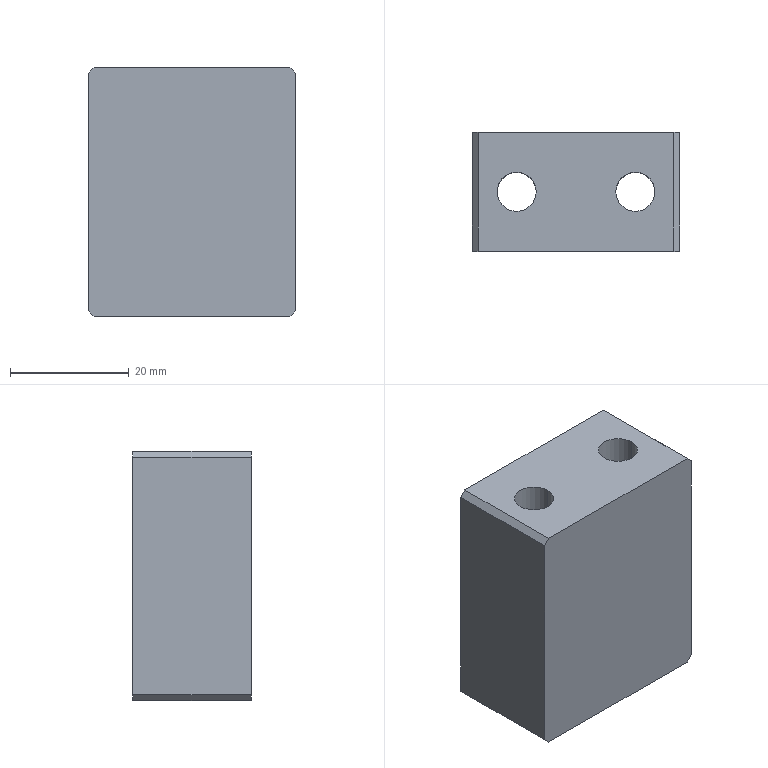Part | SolidWorks | features BaseBody 1 | 1 solid | 20 faces | box 35 x 20 x 42 mm | volume 25659 mm3 | plane 12 | cylinder 8 | commonest cylinder face diameters 6.6 x4 11 x4
STEP:
#1=CARTESIAN_POINT('',(-16.5,10.,-21.));
#2=VERTEX_POINT('',#1);
#3=CARTESIAN_POINT('',(-17.5,10.,-20.));
#4=VERTEX_POINT('',#3);
#5=CARTESIAN_POINT('',(-17.5,10.,-20.));
#6=DIRECTION('',(-0.7071,0.,0.7071));
#7=VECTOR('',#6,1000.);
#8=LINE('',#5,#7);
#9=EDGE_CURVE('',#2,#4,#8,.T.);
#10=ORIENTED_EDGE('',*,*,#9,.F.);
#11=CARTESIAN_POINT('',(-16.5,-10.,-21.));
#12=VERTEX_POINT('',#11);
#13=CARTESIAN_POINT('',(-16.5,10.,-21.));
#14=DIRECTION('',(0.,1.,0.));
#15=VECTOR('',#14,1000.);
#16=LINE('',#13,#15);
#17=EDGE_CURVE('',#12,#2,#16,.T.);
#18=ORIENTED_EDGE('',*,*,#17,.F.);
#19=CARTESIAN_POINT('',(-17.5,-10.,-20.));
#20=VERTEX_POINT('',#19);
#21=CARTESIAN_POINT('',(-18.75,-10.,-18.75));
#22=DIRECTION('',(0.7071,0.,-0.7071));
#23=VECTOR('',#22,1000.);
#24=LINE('',#21,#23);
#25=EDGE_CURVE('',#20,#12,#24,.T.);
#26=ORIENTED_EDGE('',*,*,#25,.F.);
#27=CARTESIAN_POINT('',(-17.5,10.,-20.));
#28=DIRECTION('',(0.,-1.,0.));
#29=VECTOR('',#28,1000.);
#30=LINE('',#27,#29);
#31=EDGE_CURVE('',#4,#20,#30,.T.);
#32=ORIENTED_EDGE('',*,*,#31,.F.);
#33=EDGE_LOOP('',(#10,#18,#26,#32));
#34=FACE_OUTER_BOUND('',#33,.T.);
#35=CARTESIAN_POINT('',(-17.5,10.,-20.));
#36=DIRECTION('',(0.7071,0.,0.7071));
#37=DIRECTION('',(0.,-1.,0.));
#38=AXIS2_PLACEMENT_3D('',#35,#36,#37);
#39=PLANE('',#38);
#40=ADVANCED_FACE('',(#34),#39,.F.);
#41=CARTESIAN_POINT('',(17.5,10.,-20.));
#42=VERTEX_POINT('',#41);
#43=CARTESIAN_POINT('',(16.5,10.,-21.));
#44=VERTEX_POINT('',#43);
#45=CARTESIAN_POINT('',(16.5,10.,-21.));
#46=DIRECTION('',(-0.7071,0.,-0.7071));
#47=VECTOR('',#46,1000.);
#48=LINE('',#45,#47);
#49=EDGE_CURVE('',#42,#44,#48,.T.);
#50=ORIENTED_EDGE('',*,*,#49,.F.);
#51=CARTESIAN_POINT('',(17.5,-10.,-20.));
#52=VERTEX_POINT('',#51);
#53=CARTESIAN_POINT('',(17.5,10.,-20.));
#54=DIRECTION('',(0.,1.,0.));
#55=VECTOR('',#54,1000.);
#56=LINE('',#53,#55);
#57=EDGE_CURVE('',#52,#42,#56,.T.);
#58=ORIENTED_EDGE('',*,*,#57,.F.);
#59=CARTESIAN_POINT('',(16.5,-10.,-21.));
#60=VERTEX_POINT('',#59);
#61=CARTESIAN_POINT('',(18.75,-10.,-18.75));
#62=DIRECTION('',(0.7071,0.,0.7071));
#63=VECTOR('',#62,1000.);
#64=LINE('',#61,#63);
#65=EDGE_CURVE('',#60,#52,#64,.T.);
#66=ORIENTED_EDGE('',*,*,#65,.F.);
#67=CARTESIAN_POINT('',(16.5,10.,-21.));
#68=DIRECTION('',(0.,-1.,0.));
#69=VECTOR('',#68,1000.);
#70=LINE('',#67,#69);
#71=EDGE_CURVE('',#44,#60,#70,.T.);
#72=ORIENTED_EDGE('',*,*,#71,.F.);
#73=EDGE_LOOP('',(#50,#58,#66,#72));
#74=FACE_OUTER_BOUND('',#73,.T.);
#75=CARTESIAN_POINT('',(16.5,10.,-21.));
#76=DIRECTION('',(-0.7071,0.,0.7071));
#77=DIRECTION('',(0.,1.,0.));
#78=AXIS2_PLACEMENT_3D('',#75,#76,#77);
#79=PLANE('',#78);
#80=ADVANCED_FACE('',(#74),#79,.F.);
#81=CARTESIAN_POINT('',(-17.5,10.,20.));
#82=VERTEX_POINT('',#81);
#83=CARTESIAN_POINT('',(-16.5,10.,21.));
#84=VERTEX_POINT('',#83);
#85=CARTESIAN_POINT('',(-16.5,10.,21.));
#86=DIRECTION('',(0.7071,0.,0.7071));
#87=VECTOR('',#86,1000.);
#88=LINE('',#85,#87);
#89=EDGE_CURVE('',#82,#84,#88,.T.);
#90=ORIENTED_EDGE('',*,*,#89,.F.);
#91=CARTESIAN_POINT('',(-17.5,-10.,20.));
#92=VERTEX_POINT('',#91);
#93=CARTESIAN_POINT('',(-17.5,10.,20.));
#94=DIRECTION('',(0.,1.,0.));
#95=VECTOR('',#94,1000.);
#96=LINE('',#93,#95);
#97=EDGE_CURVE('',#92,#82,#96,.T.);
#98=ORIENTED_EDGE('',*,*,#97,.F.);
#99=CARTESIAN_POINT('',(-16.5,-10.,21.));
#100=VERTEX_POINT('',#99);
#101=CARTESIAN_POINT('',(-18.75,-10.,18.75));
#102=DIRECTION('',(-0.7071,0.,-0.7071));
#103=VECTOR('',#102,1000.);
#104=LINE('',#101,#103);
#105=EDGE_CURVE('',#100,#92,#104,.T.);
#106=ORIENTED_EDGE('',*,*,#105,.F.);
#107=CARTESIAN_POINT('',(-16.5,10.,21.));
#108=DIRECTION('',(0.,-1.,0.));
#109=VECTOR('',#108,1000.);
#110=LINE('',#107,#109);
#111=EDGE_CURVE('',#84,#100,#110,.T.);
#112=ORIENTED_EDGE('',*,*,#111,.F.);
#113=EDGE_LOOP('',(#90,#98,#106,#112));
#114=FACE_OUTER_BOUND('',#113,.T.);
#115=CARTESIAN_POINT('',(-16.5,10.,21.));
#116=DIRECTION('',(0.7071,0.,-0.7071));
#117=DIRECTION('',(0.,-1.,0.));
#118=AXIS2_PLACEMENT_3D('',#115,#116,#117);
#119=PLANE('',#118);
#120=ADVANCED_FACE('',(#114),#119,.F.);
#121=CARTESIAN_POINT('',(16.5,10.,21.));
#122=VERTEX_POINT('',#121);
#123=CARTESIAN_POINT('',(17.5,10.,20.));
#124=VERTEX_POINT('',#123);
#125=CARTESIAN_POINT('',(17.5,10.,20.));
#126=DIRECTION('',(0.7071,0.,-0.7071));
#127=VECTOR('',#126,1000.);
#128=LINE('',#125,#127);
#129=EDGE_CURVE('',#122,#124,#128,.T.);
#130=ORIENTED_EDGE('',*,*,#129,.F.);
#131=CARTESIAN_POINT('',(16.5,-10.,21.));
#132=VERTEX_POINT('',#131);
#133=CARTESIAN_POINT('',(16.5,10.,21.));
#134=DIRECTION('',(0.,1.,0.));
#135=VECTOR('',#134,1000.);
#136=LINE('',#133,#135);
#137=EDGE_CURVE('',#132,#122,#136,.T.);
#138=ORIENTED_EDGE('',*,*,#137,.F.);
#139=CARTESIAN_POINT('',(17.5,-10.,20.));
#140=VERTEX_POINT('',#139);
#141=CARTESIAN_POINT('',(18.75,-10.,18.75));
#142=DIRECTION('',(-0.7071,0.,0.7071));
#143=VECTOR('',#142,1000.);
#144=LINE('',#141,#143);
#145=EDGE_CURVE('',#140,#132,#144,.T.);
#146=ORIENTED_EDGE('',*,*,#145,.F.);
#147=CARTESIAN_POINT('',(17.5,10.,20.));
#148=DIRECTION('',(0.,-1.,0.));
#149=VECTOR('',#148,1000.);
#150=LINE('',#147,#149);
#151=EDGE_CURVE('',#124,#140,#150,.T.);
#152=ORIENTED_EDGE('',*,*,#151,.F.);
#153=EDGE_LOOP('',(#130,#138,#146,#152));
#154=FACE_OUTER_BOUND('',#153,.T.);
#155=CARTESIAN_POINT('',(17.5,10.,20.));
#156=DIRECTION('',(-0.7071,0.,-0.7071));
#157=DIRECTION('',(-0.7071,0.,0.7071));
#158=AXIS2_PLACEMENT_3D('',#155,#156,#157);
#159=PLANE('',#158);
#160=ADVANCED_FACE('',(#154),#159,.F.);
#161=CARTESIAN_POINT('',(-4.5,0.,-14.2));
#162=VERTEX_POINT('',#161);
#163=CARTESIAN_POINT('',(-4.5,0.,-21.));
#164=VERTEX_POINT('',#163);
#165=CARTESIAN_POINT('',(-4.5,0.,-21.));
#166=DIRECTION('',(0.,0.,-1.));
#167=VECTOR('',#166,1000.);
#168=LINE('',#165,#167);
#169=EDGE_CURVE('',#162,#164,#168,.T.);
#170=ORIENTED_EDGE('',*,*,#169,.F.);
#171=CARTESIAN_POINT('',(-15.5,0.,-14.2));
#172=VERTEX_POINT('',#171);
#173=CARTESIAN_POINT('',(-10.,0.,-14.2));
#174=DIRECTION('',(0.,0.,-1.));
#175=DIRECTION('',(-1.,0.,0.));
#176=AXIS2_PLACEMENT_3D('',#173,#174,#175);
#177=CIRCLE('',#176,5.5);
#178=EDGE_CURVE('',#172,#162,#177,.T.);
#179=ORIENTED_EDGE('',*,*,#178,.F.);
#180=CARTESIAN_POINT('',(-15.5,0.,-21.));
#181=VERTEX_POINT('',#180);
#182=CARTESIAN_POINT('',(-15.5,0.,-21.));
#183=DIRECTION('',(0.,0.,-1.));
#184=VECTOR('',#183,1000.);
#185=LINE('',#182,#184);
#186=EDGE_CURVE('',#172,#181,#185,.T.);
#187=ORIENTED_EDGE('',*,*,#186,.T.);
#188=CARTESIAN_POINT('',(-10.,0.,-21.));
#189=DIRECTION('',(0.,0.,-1.));
#190=DIRECTION('',(-1.,0.,0.));
#191=AXIS2_PLACEMENT_3D('',#188,#189,#190);
#192=CIRCLE('',#191,5.5);
#193=EDGE_CURVE('',#181,#164,#192,.T.);
#194=ORIENTED_EDGE('',*,*,#193,.T.);
#195=EDGE_LOOP('',(#170,#179,#187,#194));
#196=FACE_OUTER_BOUND('',#195,.T.);
#197=CARTESIAN_POINT('',(-10.,0.,-21.));
#198=DIRECTION('',(0.,0.,-1.));
#199=DIRECTION('',(-1.,0.,0.));
#200=AXIS2_PLACEMENT_3D('',#197,#198,#199);
#201=CYLINDRICAL_SURFACE('',#200,5.5);
#202=ADVANCED_FACE('',(#196),#201,.F.);
#203=CARTESIAN_POINT('',(-13.3,0.,-14.2));
#204=VERTEX_POINT('',#203);
#205=CARTESIAN_POINT('',(-6.7,0.,-14.2));
#206=VERTEX_POINT('',#205);
#207=CARTESIAN_POINT('',(-10.,0.,-14.2));
#208=DIRECTION('',(0.,0.,-1.));
#209=DIRECTION('',(-1.,0.,0.));
#210=AXIS2_PLACEMENT_3D('',#207,#208,#209);
#211=CIRCLE('',#210,3.3);
#212=EDGE_CURVE('',#204,#206,#211,.T.);
#213=ORIENTED_EDGE('',*,*,#212,.F.);
#214=CARTESIAN_POINT('',(-10.,0.,-14.2));
#215=DIRECTION('',(0.,0.,-1.));
#216=DIRECTION('',(-1.,0.,0.));
#217=AXIS2_PLACEMENT_3D('',#214,#215,#216);
#218=CIRCLE('',#217,3.3);
#219=EDGE_CURVE('',#206,#204,#218,.T.);
#220=ORIENTED_EDGE('',*,*,#219,.F.);
#221=EDGE_LOOP('',(#213,#220));
#222=FACE_BOUND('',#221,.T.);
#223=ORIENTED_EDGE('',*,*,#178,.T.);
#224=CARTESIAN_POINT('',(-10.,0.,-14.2));
#225=DIRECTION('',(0.,0.,-1.));
#226=DIRECTION('',(-1.,0.,0.));
#227=AXIS2_PLACEMENT_3D('',#224,#225,#226);
#228=CIRCLE('',#227,5.5);
#229=EDGE_CURVE('',#162,#172,#228,.T.);
#230=ORIENTED_EDGE('',*,*,#229,.T.);
#231=EDGE_LOOP('',(#223,#230));
#232=FACE_OUTER_BOUND('',#231,.T.);
#233=CARTESIAN_POINT('',(-6.7,0.,-14.2));
#234=DIRECTION('',(0.,0.,1.));
#235=DIRECTION('',(1.,0.,0.));
#236=AXIS2_PLACEMENT_3D('',#233,#234,#235);
#237=PLANE('',#236);
#238=ADVANCED_FACE('',(#222,#232),#237,.F.);
#239=CARTESIAN_POINT('',(-6.7,0.,21.));
#240=VERTEX_POINT('',#239);
#241=CARTESIAN_POINT('',(-6.7,0.,-21.));
#242=DIRECTION('',(0.,0.,-1.));
#243=VECTOR('',#242,1000.);
#244=LINE('',#241,#243);
#245=EDGE_CURVE('',#240,#206,#244,.T.);
#246=ORIENTED_EDGE('',*,*,#245,.F.);
#247=CARTESIAN_POINT('',(-13.3,0.,21.));
#248=VERTEX_POINT('',#247);
#249=CARTESIAN_POINT('',(-10.,0.,21.));
#250=DIRECTION('',(0.,0.,-1.));
#251=DIRECTION('',(-1.,0.,0.));
#252=AXIS2_PLACEMENT_3D('',#249,#250,#251);
#253=CIRCLE('',#252,3.3);
#254=EDGE_CURVE('',#248,#240,#253,.T.);
#255=ORIENTED_EDGE('',*,*,#254,.F.);
#256=CARTESIAN_POINT('',(-13.3,0.,-21.));
#257=DIRECTION('',(0.,0.,-1.));
#258=VECTOR('',#257,1000.);
#259=LINE('',#256,#258);
#260=EDGE_CURVE('',#248,#204,#259,.T.);
#261=ORIENTED_EDGE('',*,*,#260,.T.);
#262=ORIENTED_EDGE('',*,*,#212,.T.);
#263=EDGE_LOOP('',(#246,#255,#261,#262));
#264=FACE_OUTER_BOUND('',#263,.T.);
#265=CARTESIAN_POINT('',(-10.,0.,-21.));
#266=DIRECTION('',(0.,0.,-1.));
#267=DIRECTION('',(-1.,0.,0.));
#268=AXIS2_PLACEMENT_3D('',#265,#266,#267);
#269=CYLINDRICAL_SURFACE('',#268,3.3);
#270=ADVANCED_FACE('',(#264),#269,.F.);
#271=CARTESIAN_POINT('',(15.5,0.,-14.2));
#272=VERTEX_POINT('',#271);
#273=CARTESIAN_POINT('',(15.5,0.,-21.));
#274=VERTEX_POINT('',#273);
#275=CARTESIAN_POINT('',(15.5,0.,-21.));
#276=DIRECTION('',(0.,0.,-1.));
#277=VECTOR('',#276,1000.);
#278=LINE('',#275,#277);
#279=EDGE_CURVE('',#272,#274,#278,.T.);
#280=ORIENTED_EDGE('',*,*,#279,.F.);
#281=CARTESIAN_POINT('',(4.5,0.,-14.2));
#282=VERTEX_POINT('',#281);
#283=CARTESIAN_POINT('',(10.,0.,-14.2));
#284=DIRECTION('',(0.,0.,-1.));
#285=DIRECTION('',(-1.,0.,0.));
#286=AXIS2_PLACEMENT_3D('',#283,#284,#285);
#287=CIRCLE('',#286,5.5);
#288=EDGE_CURVE('',#282,#272,#287,.T.);
#289=ORIENTED_EDGE('',*,*,#288,.F.);
#290=CARTESIAN_POINT('',(4.5,0.,-21.));
#291=VERTEX_POINT('',#290);
#292=CARTESIAN_POINT('',(4.5,0.,-21.));
#293=DIRECTION('',(0.,0.,-1.));
#294=VECTOR('',#293,1000.);
#295=LINE('',#292,#294);
#296=EDGE_CURVE('',#282,#291,#295,.T.);
#297=ORIENTED_EDGE('',*,*,#296,.T.);
#298=CARTESIAN_POINT('',(10.,0.,-21.));
#299=DIRECTION('',(0.,0.,-1.));
#300=DIRECTION('',(-1.,0.,0.));
#301=AXIS2_PLACEMENT_3D('',#298,#299,#300);
#302=CIRCLE('',#301,5.5);
#303=EDGE_CURVE('',#291,#274,#302,.T.);
#304=ORIENTED_EDGE('',*,*,#303,.T.);
#305=EDGE_LOOP('',(#280,#289,#297,#304));
#306=FACE_OUTER_BOUND('',#305,.T.);
#307=CARTESIAN_POINT('',(10.,0.,-21.));
#308=DIRECTION('',(0.,0.,-1.));
#309=DIRECTION('',(-1.,0.,0.));
#310=AXIS2_PLACEMENT_3D('',#307,#308,#309);
#311=CYLINDRICAL_SURFACE('',#310,5.5);
#312=ADVANCED_FACE('',(#306),#311,.F.);
#313=CARTESIAN_POINT('',(6.7,0.,-14.2));
#314=VERTEX_POINT('',#313);
#315=CARTESIAN_POINT('',(13.3,0.,-14.2));
#316=VERTEX_POINT('',#315);
#317=CARTESIAN_POINT('',(10.,0.,-14.2));
#318=DIRECTION('',(0.,0.,-1.));
#319=DIRECTION('',(-1.,0.,0.));
#320=AXIS2_PLACEMENT_3D('',#317,#318,#319);
#321=CIRCLE('',#320,3.3);
#322=EDGE_CURVE('',#314,#316,#321,.T.);
#323=ORIENTED_EDGE('',*,*,#322,.F.);
#324=CARTESIAN_POINT('',(10.,0.,-14.2));
#325=DIRECTION('',(0.,0.,-1.));
#326=DIRECTION('',(-1.,0.,0.));
#327=AXIS2_PLACEMENT_3D('',#324,#325,#326);
#328=CIRCLE('',#327,3.3);
#329=EDGE_CURVE('',#316,#314,#328,.T.);
#330=ORIENTED_EDGE('',*,*,#329,.F.);
#331=EDGE_LOOP('',(#323,#330));
#332=FACE_BOUND('',#331,.T.);
#333=ORIENTED_EDGE('',*,*,#288,.T.);
#334=CARTESIAN_POINT('',(10.,0.,-14.2));
#335=DIRECTION('',(0.,0.,-1.));
#336=DIRECTION('',(-1.,0.,0.));
#337=AXIS2_PLACEMENT_3D('',#334,#335,#336);
#338=CIRCLE('',#337,5.5);
#339=EDGE_CURVE('',#272,#282,#338,.T.);
#340=ORIENTED_EDGE('',*,*,#339,.T.);
#341=EDGE_LOOP('',(#333,#340));
#342=FACE_OUTER_BOUND('',#341,.T.);
#343=CARTESIAN_POINT('',(13.3,0.,-14.2));
#344=DIRECTION('',(0.,0.,1.));
#345=DIRECTION('',(1.,0.,0.));
#346=AXIS2_PLACEMENT_3D('',#343,#344,#345);
#347=PLANE('',#346);
#348=ADVANCED_FACE('',(#332,#342),#347,.F.);
#349=CARTESIAN_POINT('',(13.3,0.,21.));
#350=VERTEX_POINT('',#349);
#351=CARTESIAN_POINT('',(13.3,0.,-21.));
#352=DIRECTION('',(0.,0.,-1.));
#353=VECTOR('',#352,1000.);
#354=LINE('',#351,#353);
#355=EDGE_CURVE('',#350,#316,#354,.T.);
#356=ORIENTED_EDGE('',*,*,#355,.F.);
#357=CARTESIAN_POINT('',(6.7,0.,21.));
#358=VERTEX_POINT('',#357);
#359=CARTESIAN_POINT('',(10.,0.,21.));
#360=DIRECTION('',(0.,0.,-1.));
#361=DIRECTION('',(-1.,0.,0.));
#362=AXIS2_PLACEMENT_3D('',#359,#360,#361);
#363=CIRCLE('',#362,3.3);
#364=EDGE_CURVE('',#358,#350,#363,.T.);
#365=ORIENTED_EDGE('',*,*,#364,.F.);
#366=CARTESIAN_POINT('',(6.7,0.,-21.));
#367=DIRECTION('',(0.,0.,-1.));
#368=VECTOR('',#367,1000.);
#369=LINE('',#366,#368);
#370=EDGE_CURVE('',#358,#314,#369,.T.);
#371=ORIENTED_EDGE('',*,*,#370,.T.);
#372=ORIENTED_EDGE('',*,*,#322,.T.);
#373=EDGE_LOOP('',(#356,#365,#371,#372));
#374=FACE_OUTER_BOUND('',#373,.T.);
#375=CARTESIAN_POINT('',(10.,0.,-21.));
#376=DIRECTION('',(0.,0.,-1.));
#377=DIRECTION('',(-1.,0.,0.));
#378=AXIS2_PLACEMENT_3D('',#375,#376,#377);
#379=CYLINDRICAL_SURFACE('',#378,3.3);
#380=ADVANCED_FACE('',(#374),#379,.F.);
#381=CARTESIAN_POINT('',(17.5,-10.,21.));
#382=DIRECTION('',(0.,0.,-1.));
#383=VECTOR('',#382,1000.);
#384=LINE('',#381,#383);
#385=EDGE_CURVE('',#140,#52,#384,.T.);
#386=ORIENTED_EDGE('',*,*,#385,.F.);
#387=ORIENTED_EDGE('',*,*,#145,.T.);
#388=CARTESIAN_POINT('',(-17.5,-10.,21.));
#389=DIRECTION('',(1.,0.,0.));
#390=VECTOR('',#389,1000.);
#391=LINE('',#388,#390);
#392=EDGE_CURVE('',#100,#132,#391,.T.);
#393=ORIENTED_EDGE('',*,*,#392,.F.);
#394=ORIENTED_EDGE('',*,*,#105,.T.);
#395=CARTESIAN_POINT('',(-17.5,-10.,21.));
#396=DIRECTION('',(0.,0.,1.));
#397=VECTOR('',#396,1000.);
#398=LINE('',#395,#397);
#399=EDGE_CURVE('',#20,#92,#398,.T.);
#400=ORIENTED_EDGE('',*,*,#399,.F.);
#401=ORIENTED_EDGE('',*,*,#25,.T.);
#402=CARTESIAN_POINT('',(-17.5,-10.,-21.));
#403=DIRECTION('',(-1.,0.,0.));
#404=VECTOR('',#403,1000.);
#405=LINE('',#402,#404);
#406=EDGE_CURVE('',#60,#12,#405,.T.);
#407=ORIENTED_EDGE('',*,*,#406,.F.);
#408=ORIENTED_EDGE('',*,*,#65,.T.);
#409=EDGE_LOOP('',(#386,#387,#393,#394,#400,#401,#407,#408));
#410=FACE_OUTER_BOUND('',#409,.T.);
#411=CARTESIAN_POINT('',(0.,-10.,0.));
#412=DIRECTION('',(0.,-1.,0.));
#413=DIRECTION('',(0.,0.,-1.));
#414=AXIS2_PLACEMENT_3D('',#411,#412,#413);
#415=PLANE('',#414);
#416=ADVANCED_FACE('',(#410),#415,.T.);
#417=CARTESIAN_POINT('',(-17.5,10.,21.));
#418=DIRECTION('',(1.,0.,0.));
#419=VECTOR('',#418,1000.);
#420=LINE('',#417,#419);
#421=EDGE_CURVE('',#84,#122,#420,.T.);
#422=ORIENTED_EDGE('',*,*,#421,.T.);
#423=ORIENTED_EDGE('',*,*,#129,.T.);
#424=CARTESIAN_POINT('',(17.5,10.,21.));
#425=DIRECTION('',(0.,0.,-1.));
#426=VECTOR('',#425,1000.);
#427=LINE('',#424,#426);
#428=EDGE_CURVE('',#124,#42,#427,.T.);
#429=ORIENTED_EDGE('',*,*,#428,.T.);
#430=ORIENTED_EDGE('',*,*,#49,.T.);
#431=CARTESIAN_POINT('',(-17.5,10.,-21.));
#432=DIRECTION('',(-1.,0.,0.));
#433=VECTOR('',#432,1000.);
#434=LINE('',#431,#433);
#435=EDGE_CURVE('',#44,#2,#434,.T.);
#436=ORIENTED_EDGE('',*,*,#435,.T.);
#437=ORIENTED_EDGE('',*,*,#9,.T.);
#438=CARTESIAN_POINT('',(-17.5,10.,21.));
#439=DIRECTION('',(0.,0.,1.));
#440=VECTOR('',#439,1000.);
#441=LINE('',#438,#440);
#442=EDGE_CURVE('',#4,#82,#441,.T.);
#443=ORIENTED_EDGE('',*,*,#442,.T.);
#444=ORIENTED_EDGE('',*,*,#89,.T.);
#445=EDGE_LOOP('',(#422,#423,#429,#430,#436,#437,#443,#444));
#446=FACE_OUTER_BOUND('',#445,.T.);
#447=CARTESIAN_POINT('',(0.,10.,0.));
#448=DIRECTION('',(0.,-1.,0.));
#449=DIRECTION('',(0.,0.,-1.));
#450=AXIS2_PLACEMENT_3D('',#447,#448,#449);
#451=PLANE('',#450);
#452=ADVANCED_FACE('',(#446),#451,.F.);
#453=ORIENTED_EDGE('',*,*,#364,.T.);
#454=CARTESIAN_POINT('',(10.,0.,21.));
#455=DIRECTION('',(0.,0.,-1.));
#456=DIRECTION('',(-1.,0.,0.));
#457=AXIS2_PLACEMENT_3D('',#454,#455,#456);
#458=CIRCLE('',#457,3.3);
#459=EDGE_CURVE('',#350,#358,#458,.T.);
#460=ORIENTED_EDGE('',*,*,#459,.T.);
#461=EDGE_LOOP('',(#453,#460));
#462=FACE_BOUND('',#461,.T.);
#463=ORIENTED_EDGE('',*,*,#254,.T.);
#464=CARTESIAN_POINT('',(-10.,0.,21.));
#465=DIRECTION('',(0.,0.,-1.));
#466=DIRECTION('',(-1.,0.,0.));
#467=AXIS2_PLACEMENT_3D('',#464,#465,#466);
#468=CIRCLE('',#467,3.3);
#469=EDGE_CURVE('',#240,#248,#468,.T.);
#470=ORIENTED_EDGE('',*,*,#469,.T.);
#471=EDGE_LOOP('',(#463,#470));
#472=FACE_BOUND('',#471,.T.);
#473=ORIENTED_EDGE('',*,*,#392,.T.);
#474=ORIENTED_EDGE('',*,*,#137,.T.);
#475=ORIENTED_EDGE('',*,*,#421,.F.);
#476=ORIENTED_EDGE('',*,*,#111,.T.);
#477=EDGE_LOOP('',(#473,#474,#475,#476));
#478=FACE_OUTER_BOUND('',#477,.T.);
#479=CARTESIAN_POINT('',(-17.5,10.,21.));
#480=DIRECTION('',(0.,0.,-1.));
#481=DIRECTION('',(0.,-1.,0.));
#482=AXIS2_PLACEMENT_3D('',#479,#480,#481);
#483=PLANE('',#482);
#484=ADVANCED_FACE('',(#462,#472,#478),#483,.F.);
#485=ORIENTED_EDGE('',*,*,#399,.T.);
#486=ORIENTED_EDGE('',*,*,#97,.T.);
#487=ORIENTED_EDGE('',*,*,#442,.F.);
#488=ORIENTED_EDGE('',*,*,#31,.T.);
#489=EDGE_LOOP('',(#485,#486,#487,#488));
#490=FACE_OUTER_BOUND('',#489,.T.);
#491=CARTESIAN_POINT('',(-17.5,10.,21.));
#492=DIRECTION('',(1.,0.,0.));
#493=DIRECTION('',(0.,1.,0.));
#494=AXIS2_PLACEMENT_3D('',#491,#492,#493);
#495=PLANE('',#494);
#496=ADVANCED_FACE('',(#490),#495,.F.);
#497=ORIENTED_EDGE('',*,*,#303,.F.);
#498=CARTESIAN_POINT('',(10.,0.,-21.));
#499=DIRECTION('',(0.,0.,-1.));
#500=DIRECTION('',(-1.,0.,0.));
#501=AXIS2_PLACEMENT_3D('',#498,#499,#500);
#502=CIRCLE('',#501,5.5);
#503=EDGE_CURVE('',#274,#291,#502,.T.);
#504=ORIENTED_EDGE('',*,*,#503,.F.);
#505=EDGE_LOOP('',(#497,#504));
#506=FACE_BOUND('',#505,.T.);
#507=ORIENTED_EDGE('',*,*,#193,.F.);
#508=CARTESIAN_POINT('',(-10.,0.,-21.));
#509=DIRECTION('',(0.,0.,-1.));
#510=DIRECTION('',(-1.,0.,0.));
#511=AXIS2_PLACEMENT_3D('',#508,#509,#510);
#512=CIRCLE('',#511,5.5);
#513=EDGE_CURVE('',#164,#181,#512,.T.);
#514=ORIENTED_EDGE('',*,*,#513,.F.);
#515=EDGE_LOOP('',(#507,#514));
#516=FACE_BOUND('',#515,.T.);
#517=ORIENTED_EDGE('',*,*,#435,.F.);
#518=ORIENTED_EDGE('',*,*,#71,.T.);
#519=ORIENTED_EDGE('',*,*,#406,.T.);
#520=ORIENTED_EDGE('',*,*,#17,.T.);
#521=EDGE_LOOP('',(#517,#518,#519,#520));
#522=FACE_OUTER_BOUND('',#521,.T.);
#523=CARTESIAN_POINT('',(-17.5,10.,-21.));
#524=DIRECTION('',(0.,0.,1.));
#525=DIRECTION('',(1.,0.,0.));
#526=AXIS2_PLACEMENT_3D('',#523,#524,#525);
#527=PLANE('',#526);
#528=ADVANCED_FACE('',(#506,#516,#522),#527,.F.);
#529=ORIENTED_EDGE('',*,*,#428,.F.);
#530=ORIENTED_EDGE('',*,*,#151,.T.);
#531=ORIENTED_EDGE('',*,*,#385,.T.);
#532=ORIENTED_EDGE('',*,*,#57,.T.);
#533=EDGE_LOOP('',(#529,#530,#531,#532));
#534=FACE_OUTER_BOUND('',#533,.T.);
#535=CARTESIAN_POINT('',(17.5,10.,21.));
#536=DIRECTION('',(-1.,0.,0.));
#537=DIRECTION('',(0.,0.,1.));
#538=AXIS2_PLACEMENT_3D('',#535,#536,#537);
#539=PLANE('',#538);
#540=ADVANCED_FACE('',(#534),#539,.F.);
#541=ORIENTED_EDGE('',*,*,#459,.F.);
#542=ORIENTED_EDGE('',*,*,#355,.T.);
#543=ORIENTED_EDGE('',*,*,#329,.T.);
#544=ORIENTED_EDGE('',*,*,#370,.F.);
#545=EDGE_LOOP('',(#541,#542,#543,#544));
#546=FACE_OUTER_BOUND('',#545,.T.);
#547=CARTESIAN_POINT('',(10.,0.,-21.));
#548=DIRECTION('',(0.,0.,-1.));
#549=DIRECTION('',(-1.,0.,0.));
#550=AXIS2_PLACEMENT_3D('',#547,#548,#549);
#551=CYLINDRICAL_SURFACE('',#550,3.3);
#552=ADVANCED_FACE('',(#546),#551,.F.);
#553=ORIENTED_EDGE('',*,*,#339,.F.);
#554=ORIENTED_EDGE('',*,*,#279,.T.);
#555=ORIENTED_EDGE('',*,*,#503,.T.);
#556=ORIENTED_EDGE('',*,*,#296,.F.);
#557=EDGE_LOOP('',(#553,#554,#555,#556));
#558=FACE_OUTER_BOUND('',#557,.T.);
#559=CARTESIAN_POINT('',(10.,0.,-21.));
#560=DIRECTION('',(0.,0.,-1.));
#561=DIRECTION('',(-1.,0.,0.));
#562=AXIS2_PLACEMENT_3D('',#559,#560,#561);
#563=CYLINDRICAL_SURFACE('',#562,5.5);
#564=ADVANCED_FACE('',(#558),#563,.F.);
#565=ORIENTED_EDGE('',*,*,#469,.F.);
#566=ORIENTED_EDGE('',*,*,#245,.T.);
#567=ORIENTED_EDGE('',*,*,#219,.T.);
#568=ORIENTED_EDGE('',*,*,#260,.F.);
#569=EDGE_LOOP('',(#565,#566,#567,#568));
#570=FACE_OUTER_BOUND('',#569,.T.);
#571=CARTESIAN_POINT('',(-10.,0.,-21.));
#572=DIRECTION('',(0.,0.,-1.));
#573=DIRECTION('',(-1.,0.,0.));
#574=AXIS2_PLACEMENT_3D('',#571,#572,#573);
#575=CYLINDRICAL_SURFACE('',#574,3.3);
#576=ADVANCED_FACE('',(#570),#575,.F.);
#577=ORIENTED_EDGE('',*,*,#229,.F.);
#578=ORIENTED_EDGE('',*,*,#169,.T.);
#579=ORIENTED_EDGE('',*,*,#513,.T.);
#580=ORIENTED_EDGE('',*,*,#186,.F.);
#581=EDGE_LOOP('',(#577,#578,#579,#580));
#582=FACE_OUTER_BOUND('',#581,.T.);
#583=CARTESIAN_POINT('',(-10.,0.,-21.));
#584=DIRECTION('',(0.,0.,-1.));
#585=DIRECTION('',(-1.,0.,0.));
#586=AXIS2_PLACEMENT_3D('',#583,#584,#585);
#587=CYLINDRICAL_SURFACE('',#586,5.5);
#588=ADVANCED_FACE('',(#582),#587,.F.);
#589=CLOSED_SHELL('',(#40,#80,#120,#160,#202,#238,#270,#312,#348,#380,#416,#452,#484,#496,#528,#540,#552,#564,#576,#588));
#590=MANIFOLD_SOLID_BREP('',#589);
#591=CARTESIAN_POINT('',(0.,0.,0.));
#592=DIRECTION('',(0.,0.,1.));
#593=DIRECTION('',(1.,0.,0.));
#594=AXIS2_PLACEMENT_3D('',#591,#592,#593);
#595=(LENGTH_UNIT()NAMED_UNIT(*)SI_UNIT(.MILLI.,.METRE.));
#596=UNCERTAINTY_MEASURE_WITH_UNIT(LENGTH_MEASURE(0.00001),#595,'','');
#597=(NAMED_UNIT(*)PLANE_ANGLE_UNIT()SI_UNIT($,.RADIAN.));
#598=(NAMED_UNIT(*)SI_UNIT($,.STERADIAN.)SOLID_ANGLE_UNIT());
#599=(GEOMETRIC_REPRESENTATION_CONTEXT(3)GLOBAL_UNCERTAINTY_ASSIGNED_CONTEXT((#596))GLOBAL_UNIT_ASSIGNED_CONTEXT((#595,#597,#598))REPRESENTATION_CONTEXT('',''));
#600=ADVANCED_BREP_SHAPE_REPRESENTATION('',(#590,#594),#599);